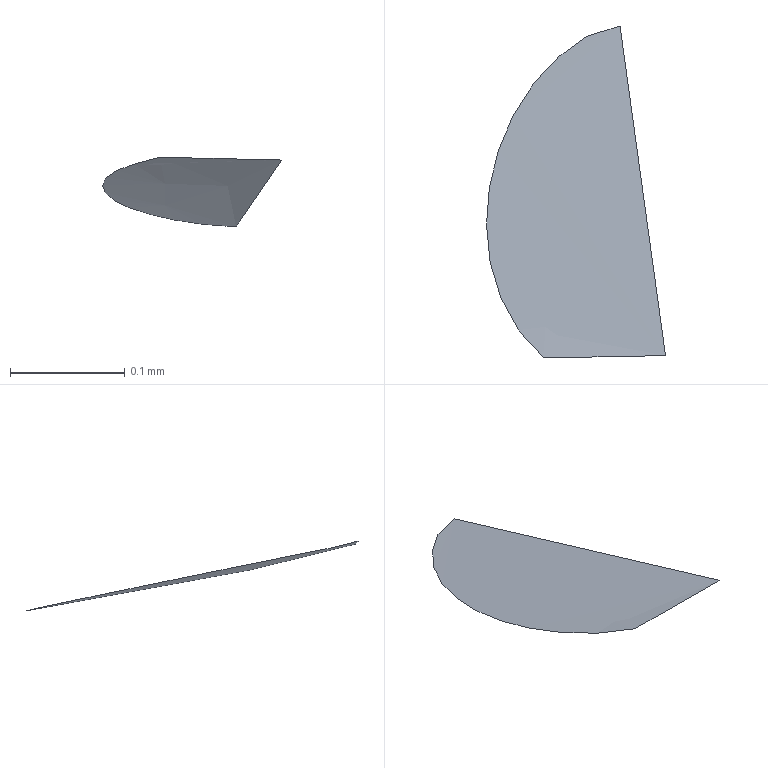Part | NX | features solid 2 | 1 solid | 2 faces | volume 0.00007157 mm3 | spline 2